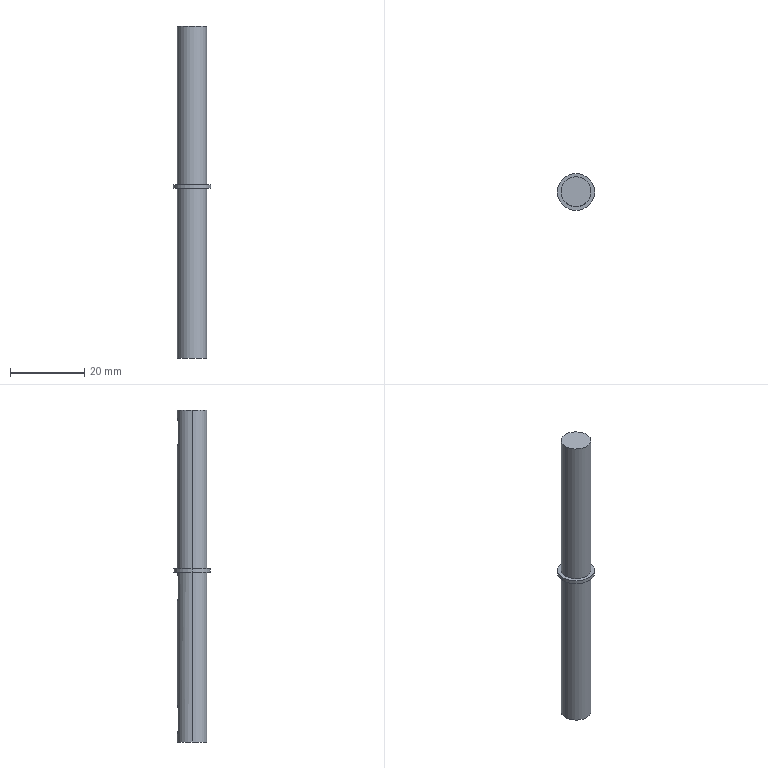Part | SolidWorks | features ICE 3, Extrusion 1 | 1 solid | 28 faces | box 10 x 10 x 89.39 mm | volume 4408 mm3 | cylinder 15 | plane 13 | commonest cylinder face diameters 3 x9 8 x4 10 x2
STEP:
#1=CARTESIAN_POINT('',(0.,2.2,10.));
#2=VERTEX_POINT('',#1);
#3=CARTESIAN_POINT('',(1.5,2.2,8.5));
#4=VERTEX_POINT('',#3);
#5=CARTESIAN_POINT('',(0.,2.2,8.5));
#6=DIRECTION('',(0.,1.,0.));
#7=DIRECTION('',(0.,0.,1.));
#8=AXIS2_PLACEMENT_3D('',#5,#6,#7);
#9=CIRCLE('',#8,1.5);
#10=EDGE_CURVE('',#2,#4,#9,.T.);
#11=ORIENTED_EDGE('',*,*,#10,.F.);
#12=CARTESIAN_POINT('',(0.,4.,10.));
#13=VERTEX_POINT('',#12);
#14=CARTESIAN_POINT('',(0.,2.2,10.));
#15=DIRECTION('',(0.,1.,0.));
#16=VECTOR('',#15,1000.);
#17=LINE('',#14,#16);
#18=EDGE_CURVE('',#2,#13,#17,.T.);
#19=ORIENTED_EDGE('',*,*,#18,.T.);
#20=CARTESIAN_POINT('',(1.5,3.708,8.5));
#21=VERTEX_POINT('',#20);
#22=CARTESIAN_POINT('',(1.5,3.708,8.5));
#23=CARTESIAN_POINT('',(1.5,3.708,8.6));
#24=CARTESIAN_POINT('',(1.49,3.712,8.698));
#25=CARTESIAN_POINT('',(1.451,3.727,8.891));
#26=CARTESIAN_POINT('',(1.422,3.739,8.987));
#27=CARTESIAN_POINT('',(1.309,3.781,9.259));
#28=CARTESIAN_POINT('',(1.197,3.819,9.424));
#29=CARTESIAN_POINT('',(0.9232,3.895,9.698));
#30=CARTESIAN_POINT('',(0.7573,3.932,9.809));
#31=CARTESIAN_POINT('',(0.4867,3.971,9.922));
#32=CARTESIAN_POINT('',(0.3912,3.982,9.951));
#33=CARTESIAN_POINT('',(0.197,3.996,9.99));
#34=CARTESIAN_POINT('',(0.09895,4.,10.));
#35=CARTESIAN_POINT('',(0.,4.,10.));
#36=B_SPLINE_CURVE_WITH_KNOTS('',3,(#22,#23,#24,#25,#26,#27,#28,#29,#30,#31,#32,#33,#34,#35),.UNSPECIFIED.,.F.,.F.,(4,2,2,2,2,2,4),(0.,0.0002959,0.0005918,0.001184,0.001775,0.002071,0.002367),.UNSPECIFIED.);
#37=EDGE_CURVE('',#21,#13,#36,.T.);
#38=ORIENTED_EDGE('',*,*,#37,.F.);
#39=CARTESIAN_POINT('',(1.5,2.2,8.5));
#40=DIRECTION('',(0.,1.,0.));
#41=VECTOR('',#40,1000.);
#42=LINE('',#39,#41);
#43=EDGE_CURVE('',#4,#21,#42,.T.);
#44=ORIENTED_EDGE('',*,*,#43,.F.);
#45=EDGE_LOOP('',(#11,#19,#38,#44));
#46=FACE_OUTER_BOUND('',#45,.T.);
#47=CARTESIAN_POINT('',(0.,2.2,8.5));
#48=DIRECTION('',(0.,1.,0.));
#49=DIRECTION('',(0.,0.,1.));
#50=AXIS2_PLACEMENT_3D('',#47,#48,#49);
#51=CYLINDRICAL_SURFACE('',#50,1.5);
#52=ADVANCED_FACE('',(#46),#51,.F.);
#53=CARTESIAN_POINT('',(0.,2.2,45.65));
#54=VERTEX_POINT('',#53);
#55=CARTESIAN_POINT('',(1.5,2.2,44.15));
#56=VERTEX_POINT('',#55);
#57=CARTESIAN_POINT('',(0.,2.2,44.15));
#58=DIRECTION('',(0.,1.,0.));
#59=DIRECTION('',(0.,0.,1.));
#60=AXIS2_PLACEMENT_3D('',#57,#58,#59);
#61=CIRCLE('',#60,1.5);
#62=EDGE_CURVE('',#54,#56,#61,.T.);
#63=ORIENTED_EDGE('',*,*,#62,.F.);
#64=CARTESIAN_POINT('',(0.,4.,45.65));
#65=VERTEX_POINT('',#64);
#66=CARTESIAN_POINT('',(0.,2.2,45.65));
#67=DIRECTION('',(0.,1.,0.));
#68=VECTOR('',#67,1000.);
#69=LINE('',#66,#68);
#70=EDGE_CURVE('',#54,#65,#69,.T.);
#71=ORIENTED_EDGE('',*,*,#70,.T.);
#72=CARTESIAN_POINT('',(1.5,3.708,44.15));
#73=VERTEX_POINT('',#72);
#74=CARTESIAN_POINT('',(1.5,3.708,44.15));
#75=CARTESIAN_POINT('',(1.5,3.708,44.25));
#76=CARTESIAN_POINT('',(1.49,3.712,44.348));
#77=CARTESIAN_POINT('',(1.451,3.727,44.541));
#78=CARTESIAN_POINT('',(1.422,3.739,44.637));
#79=CARTESIAN_POINT('',(1.309,3.781,44.909));
#80=CARTESIAN_POINT('',(1.197,3.819,45.074));
#81=CARTESIAN_POINT('',(0.9232,3.895,45.348));
#82=CARTESIAN_POINT('',(0.7573,3.932,45.459));
#83=CARTESIAN_POINT('',(0.4867,3.971,45.572));
#84=CARTESIAN_POINT('',(0.3912,3.982,45.601));
#85=CARTESIAN_POINT('',(0.197,3.996,45.64));
#86=CARTESIAN_POINT('',(0.09895,4.,45.65));
#87=CARTESIAN_POINT('',(0.,4.,45.65));
#88=B_SPLINE_CURVE_WITH_KNOTS('',3,(#74,#75,#76,#77,#78,#79,#80,#81,#82,#83,#84,#85,#86,#87),.UNSPECIFIED.,.F.,.F.,(4,2,2,2,2,2,4),(0.,0.0002959,0.0005918,0.001184,0.001775,0.002071,0.002367),.UNSPECIFIED.);
#89=EDGE_CURVE('',#73,#65,#88,.T.);
#90=ORIENTED_EDGE('',*,*,#89,.F.);
#91=CARTESIAN_POINT('',(1.5,2.2,44.15));
#92=DIRECTION('',(0.,1.,0.));
#93=VECTOR('',#92,1000.);
#94=LINE('',#91,#93);
#95=EDGE_CURVE('',#56,#73,#94,.T.);
#96=ORIENTED_EDGE('',*,*,#95,.F.);
#97=EDGE_LOOP('',(#63,#71,#90,#96));
#98=FACE_OUTER_BOUND('',#97,.T.);
#99=CARTESIAN_POINT('',(0.,2.2,44.15));
#100=DIRECTION('',(0.,1.,0.));
#101=DIRECTION('',(0.,0.,1.));
#102=AXIS2_PLACEMENT_3D('',#99,#100,#101);
#103=CYLINDRICAL_SURFACE('',#102,1.5);
#104=ADVANCED_FACE('',(#98),#103,.F.);
#105=CARTESIAN_POINT('',(0.,2.2,87.39));
#106=VERTEX_POINT('',#105);
#107=CARTESIAN_POINT('',(1.5,2.2,85.89));
#108=VERTEX_POINT('',#107);
#109=CARTESIAN_POINT('',(0.,2.2,85.89));
#110=DIRECTION('',(0.,1.,0.));
#111=DIRECTION('',(0.,0.,1.));
#112=AXIS2_PLACEMENT_3D('',#109,#110,#111);
#113=CIRCLE('',#112,1.5);
#114=EDGE_CURVE('',#106,#108,#113,.T.);
#115=ORIENTED_EDGE('',*,*,#114,.F.);
#116=CARTESIAN_POINT('',(0.,4.,87.39));
#117=VERTEX_POINT('',#116);
#118=CARTESIAN_POINT('',(0.,2.2,87.39));
#119=DIRECTION('',(0.,1.,0.));
#120=VECTOR('',#119,1000.);
#121=LINE('',#118,#120);
#122=EDGE_CURVE('',#106,#117,#121,.T.);
#123=ORIENTED_EDGE('',*,*,#122,.T.);
#124=CARTESIAN_POINT('',(1.5,3.708,85.89));
#125=VERTEX_POINT('',#124);
#126=CARTESIAN_POINT('',(1.5,3.708,85.89));
#127=CARTESIAN_POINT('',(1.5,3.708,85.99));
#128=CARTESIAN_POINT('',(1.49,3.712,86.088));
#129=CARTESIAN_POINT('',(1.451,3.727,86.281));
#130=CARTESIAN_POINT('',(1.422,3.739,86.377));
#131=CARTESIAN_POINT('',(1.309,3.781,86.649));
#132=CARTESIAN_POINT('',(1.197,3.819,86.814));
#133=CARTESIAN_POINT('',(0.9232,3.895,87.088));
#134=CARTESIAN_POINT('',(0.7573,3.932,87.199));
#135=CARTESIAN_POINT('',(0.4867,3.971,87.312));
#136=CARTESIAN_POINT('',(0.3912,3.982,87.341));
#137=CARTESIAN_POINT('',(0.197,3.996,87.38));
#138=CARTESIAN_POINT('',(0.09895,4.,87.39));
#139=CARTESIAN_POINT('',(0.,4.,87.39));
#140=B_SPLINE_CURVE_WITH_KNOTS('',3,(#126,#127,#128,#129,#130,#131,#132,#133,#134,#135,#136,#137,#138,#139),.UNSPECIFIED.,.F.,.F.,(4,2,2,2,2,2,4),(0.,0.0002959,0.0005918,0.001184,0.001775,0.002071,0.002367),.UNSPECIFIED.);
#141=EDGE_CURVE('',#125,#117,#140,.T.);
#142=ORIENTED_EDGE('',*,*,#141,.F.);
#143=CARTESIAN_POINT('',(1.5,2.2,85.89));
#144=DIRECTION('',(0.,1.,0.));
#145=VECTOR('',#144,1000.);
#146=LINE('',#143,#145);
#147=EDGE_CURVE('',#108,#125,#146,.T.);
#148=ORIENTED_EDGE('',*,*,#147,.F.);
#149=EDGE_LOOP('',(#115,#123,#142,#148));
#150=FACE_OUTER_BOUND('',#149,.T.);
#151=CARTESIAN_POINT('',(0.,2.2,85.89));
#152=DIRECTION('',(0.,1.,0.));
#153=DIRECTION('',(0.,0.,1.));
#154=AXIS2_PLACEMENT_3D('',#151,#152,#153);
#155=CYLINDRICAL_SURFACE('',#154,1.5);
#156=ADVANCED_FACE('',(#150),#155,.F.);
#157=CARTESIAN_POINT('',(1.5,3.708,80.89));
#158=VERTEX_POINT('',#157);
#159=CARTESIAN_POINT('',(1.5,3.708,89.39));
#160=DIRECTION('',(0.,0.,1.));
#161=VECTOR('',#160,1000.);
#162=LINE('',#159,#161);
#163=EDGE_CURVE('',#158,#125,#162,.T.);
#164=ORIENTED_EDGE('',*,*,#163,.T.);
#165=ORIENTED_EDGE('',*,*,#141,.T.);
#166=CARTESIAN_POINT('',(-1.5,3.708,85.89));
#167=VERTEX_POINT('',#166);
#168=CARTESIAN_POINT('',(0.,4.,87.39));
#169=CARTESIAN_POINT('',(-0.0988,4.,87.39));
#170=CARTESIAN_POINT('',(-0.1991,3.996,87.38));
#171=CARTESIAN_POINT('',(-0.3921,3.982,87.341));
#172=CARTESIAN_POINT('',(-0.486,3.971,87.313));
#173=CARTESIAN_POINT('',(-0.6687,3.945,87.236));
#174=CARTESIAN_POINT('',(-0.7547,3.929,87.19));
#175=CARTESIAN_POINT('',(-0.9162,3.895,87.082));
#176=CARTESIAN_POINT('',(-0.9924,3.876,87.019));
#177=CARTESIAN_POINT('',(-1.13,3.838,86.881));
#178=CARTESIAN_POINT('',(-1.191,3.819,86.807));
#179=CARTESIAN_POINT('',(-1.3,3.783,86.645));
#180=CARTESIAN_POINT('',(-1.347,3.767,86.558));
#181=CARTESIAN_POINT('',(-1.459,3.725,86.288));
#182=CARTESIAN_POINT('',(-1.5,3.708,86.09));
#183=CARTESIAN_POINT('',(-1.5,3.708,85.89));
#184=B_SPLINE_CURVE_WITH_KNOTS('',3,(#168,#169,#170,#171,#172,#173,#174,#175,#176,#177,#178,#179,#180,#181,#182,#183),.UNSPECIFIED.,.F.,.F.,(4,2,2,2,2,2,2,4),(0.002367,0.002663,0.002958,0.003254,0.003549,0.003845,0.00414,0.004731),.UNSPECIFIED.);
#185=EDGE_CURVE('',#117,#167,#184,.T.);
#186=ORIENTED_EDGE('',*,*,#185,.T.);
#187=CARTESIAN_POINT('',(-1.5,3.708,80.89));
#188=VERTEX_POINT('',#187);
#189=CARTESIAN_POINT('',(-1.5,3.708,89.39));
#190=DIRECTION('',(0.,0.,-1.));
#191=VECTOR('',#190,1000.);
#192=LINE('',#189,#191);
#193=EDGE_CURVE('',#167,#188,#192,.T.);
#194=ORIENTED_EDGE('',*,*,#193,.T.);
#195=CARTESIAN_POINT('',(-1.5,3.708,80.89));
#196=CARTESIAN_POINT('',(-1.5,3.708,80.79));
#197=CARTESIAN_POINT('',(-1.49,3.712,80.692));
#198=CARTESIAN_POINT('',(-1.451,3.727,80.499));
#199=CARTESIAN_POINT('',(-1.422,3.739,80.403));
#200=CARTESIAN_POINT('',(-1.309,3.781,80.132));
#201=CARTESIAN_POINT('',(-1.198,3.819,79.967));
#202=CARTESIAN_POINT('',(-0.924,3.894,79.693));
#203=CARTESIAN_POINT('',(-0.7582,3.932,79.581));
#204=CARTESIAN_POINT('',(-0.488,3.971,79.468));
#205=CARTESIAN_POINT('',(-0.3926,3.982,79.439));
#206=CARTESIAN_POINT('',(-0.1986,3.996,79.4));
#207=CARTESIAN_POINT('',(-0.1006,4.,79.39));
#208=CARTESIAN_POINT('',(0.09712,4.,79.39));
#209=CARTESIAN_POINT('',(0.1975,3.996,79.4));
#210=CARTESIAN_POINT('',(0.3907,3.982,79.438));
#211=CARTESIAN_POINT('',(0.4847,3.972,79.467));
#212=CARTESIAN_POINT('',(0.759,3.932,79.581));
#213=CARTESIAN_POINT('',(0.9229,3.895,79.692));
#214=CARTESIAN_POINT('',(1.129,3.838,79.898));
#215=CARTESIAN_POINT('',(1.191,3.819,79.973));
#216=CARTESIAN_POINT('',(1.299,3.783,80.134));
#217=CARTESIAN_POINT('',(1.347,3.767,80.222));
#218=CARTESIAN_POINT('',(1.459,3.725,80.492));
#219=CARTESIAN_POINT('',(1.5,3.708,80.69));
#220=CARTESIAN_POINT('',(1.5,3.708,80.89));
#221=B_SPLINE_CURVE_WITH_KNOTS('',3,(#195,#196,#197,#198,#199,#200,#201,#202,#203,#204,#205,#206,#207,#208,#209,#210,#211,#212,#213,#214,#215,#216,#217,#218,#219,#220),.UNSPECIFIED.,.F.,.F.,(4,2,2,2,2,2,2,2,2,2,2,2,4),(0.,0.0002957,0.0005914,0.001183,0.001774,0.00207,0.002366,0.002661,0.002957,0.003548,0.003844,0.00414,0.004731),.UNSPECIFIED.);
#222=EDGE_CURVE('',#188,#158,#221,.T.);
#223=ORIENTED_EDGE('',*,*,#222,.T.);
#224=EDGE_LOOP('',(#164,#165,#186,#194,#223));
#225=FACE_BOUND('',#224,.T.);
#226=CARTESIAN_POINT('',(4.,0.,89.39));
#227=VERTEX_POINT('',#226);
#228=CARTESIAN_POINT('',(-4.,0.,89.39));
#229=VERTEX_POINT('',#228);
#230=CARTESIAN_POINT('',(0.,0.,89.39));
#231=DIRECTION('',(0.,0.,1.));
#232=DIRECTION('',(1.,0.,0.));
#233=AXIS2_PLACEMENT_3D('',#230,#231,#232);
#234=CIRCLE('',#233,4.);
#235=EDGE_CURVE('',#227,#229,#234,.T.);
#236=ORIENTED_EDGE('',*,*,#235,.F.);
#237=CARTESIAN_POINT('',(4.,0.,46.65));
#238=VERTEX_POINT('',#237);
#239=CARTESIAN_POINT('',(4.,0.,89.39));
#240=DIRECTION('',(0.,0.,-1.));
#241=VECTOR('',#240,1000.);
#242=LINE('',#239,#241);
#243=EDGE_CURVE('',#227,#238,#242,.T.);
#244=ORIENTED_EDGE('',*,*,#243,.T.);
#245=CARTESIAN_POINT('',(-4.,0.,46.65));
#246=VERTEX_POINT('',#245);
#247=CARTESIAN_POINT('',(0.,0.,46.65));
#248=DIRECTION('',(0.,0.,1.));
#249=DIRECTION('',(1.,0.,0.));
#250=AXIS2_PLACEMENT_3D('',#247,#248,#249);
#251=CIRCLE('',#250,4.);
#252=EDGE_CURVE('',#238,#246,#251,.T.);
#253=ORIENTED_EDGE('',*,*,#252,.T.);
#254=CARTESIAN_POINT('',(-4.,0.,89.39));
#255=DIRECTION('',(0.,0.,-1.));
#256=VECTOR('',#255,1000.);
#257=LINE('',#254,#256);
#258=EDGE_CURVE('',#229,#246,#257,.T.);
#259=ORIENTED_EDGE('',*,*,#258,.F.);
#260=EDGE_LOOP('',(#236,#244,#253,#259));
#261=FACE_OUTER_BOUND('',#260,.T.);
#262=CARTESIAN_POINT('',(0.,0.,89.39));
#263=DIRECTION('',(0.,0.,-1.));
#264=DIRECTION('',(-1.,0.,0.));
#265=AXIS2_PLACEMENT_3D('',#262,#263,#264);
#266=CYLINDRICAL_SURFACE('',#265,4.);
#267=ADVANCED_FACE('',(#225,#261),#266,.T.);
#268=CARTESIAN_POINT('',(5.,0.,46.65));
#269=VERTEX_POINT('',#268);
#270=CARTESIAN_POINT('',(-5.,0.,46.65));
#271=VERTEX_POINT('',#270);
#272=CARTESIAN_POINT('',(0.,0.,46.65));
#273=DIRECTION('',(0.,0.,1.));
#274=DIRECTION('',(1.,0.,0.));
#275=AXIS2_PLACEMENT_3D('',#272,#273,#274);
#276=CIRCLE('',#275,5.);
#277=EDGE_CURVE('',#269,#271,#276,.T.);
#278=ORIENTED_EDGE('',*,*,#277,.F.);
#279=CARTESIAN_POINT('',(5.,0.,45.65));
#280=VERTEX_POINT('',#279);
#281=CARTESIAN_POINT('',(5.,0.,46.65));
#282=DIRECTION('',(0.,0.,-1.));
#283=VECTOR('',#282,1000.);
#284=LINE('',#281,#283);
#285=EDGE_CURVE('',#269,#280,#284,.T.);
#286=ORIENTED_EDGE('',*,*,#285,.T.);
#287=CARTESIAN_POINT('',(-5.,0.,45.65));
#288=VERTEX_POINT('',#287);
#289=CARTESIAN_POINT('',(0.,0.,45.65));
#290=DIRECTION('',(0.,0.,1.));
#291=DIRECTION('',(1.,0.,0.));
#292=AXIS2_PLACEMENT_3D('',#289,#290,#291);
#293=CIRCLE('',#292,5.);
#294=EDGE_CURVE('',#280,#288,#293,.T.);
#295=ORIENTED_EDGE('',*,*,#294,.T.);
#296=CARTESIAN_POINT('',(-5.,0.,46.65));
#297=DIRECTION('',(0.,0.,-1.));
#298=VECTOR('',#297,1000.);
#299=LINE('',#296,#298);
#300=EDGE_CURVE('',#271,#288,#299,.T.);
#301=ORIENTED_EDGE('',*,*,#300,.F.);
#302=EDGE_LOOP('',(#278,#286,#295,#301));
#303=FACE_OUTER_BOUND('',#302,.T.);
#304=CARTESIAN_POINT('',(0.,0.,46.65));
#305=DIRECTION('',(0.,0.,-1.));
#306=DIRECTION('',(-1.,0.,0.));
#307=AXIS2_PLACEMENT_3D('',#304,#305,#306);
#308=CYLINDRICAL_SURFACE('',#307,5.);
#309=ADVANCED_FACE('',(#303),#308,.T.);
#310=CARTESIAN_POINT('',(1.5,3.708,3.5));
#311=VERTEX_POINT('',#310);
#312=CARTESIAN_POINT('',(1.5,3.708,45.65));
#313=DIRECTION('',(0.,0.,1.));
#314=VECTOR('',#313,1000.);
#315=LINE('',#312,#314);
#316=EDGE_CURVE('',#311,#21,#315,.T.);
#317=ORIENTED_EDGE('',*,*,#316,.T.);
#318=ORIENTED_EDGE('',*,*,#37,.T.);
#319=CARTESIAN_POINT('',(-1.5,3.708,8.5));
#320=VERTEX_POINT('',#319);
#321=CARTESIAN_POINT('',(0.,4.,10.));
#322=CARTESIAN_POINT('',(-0.0988,4.,10.));
#323=CARTESIAN_POINT('',(-0.1991,3.996,9.99));
#324=CARTESIAN_POINT('',(-0.3921,3.982,9.951));
#325=CARTESIAN_POINT('',(-0.486,3.971,9.923));
#326=CARTESIAN_POINT('',(-0.6687,3.945,9.846));
#327=CARTESIAN_POINT('',(-0.7547,3.929,9.8));
#328=CARTESIAN_POINT('',(-0.9162,3.895,9.692));
#329=CARTESIAN_POINT('',(-0.9924,3.876,9.629));
#330=CARTESIAN_POINT('',(-1.13,3.838,9.491));
#331=CARTESIAN_POINT('',(-1.191,3.819,9.417));
#332=CARTESIAN_POINT('',(-1.3,3.783,9.255));
#333=CARTESIAN_POINT('',(-1.347,3.767,9.168));
#334=CARTESIAN_POINT('',(-1.459,3.725,8.898));
#335=CARTESIAN_POINT('',(-1.5,3.708,8.7));
#336=CARTESIAN_POINT('',(-1.5,3.708,8.5));
#337=B_SPLINE_CURVE_WITH_KNOTS('',3,(#321,#322,#323,#324,#325,#326,#327,#328,#329,#330,#331,#332,#333,#334,#335,#336),.UNSPECIFIED.,.F.,.F.,(4,2,2,2,2,2,2,4),(0.002367,0.002663,0.002958,0.003254,0.003549,0.003845,0.00414,0.004731),.UNSPECIFIED.);
#338=EDGE_CURVE('',#13,#320,#337,.T.);
#339=ORIENTED_EDGE('',*,*,#338,.T.);
#340=CARTESIAN_POINT('',(-1.5,3.708,3.5));
#341=VERTEX_POINT('',#340);
#342=CARTESIAN_POINT('',(-1.5,3.708,45.65));
#343=DIRECTION('',(0.,0.,-1.));
#344=VECTOR('',#343,1000.);
#345=LINE('',#342,#344);
#346=EDGE_CURVE('',#320,#341,#345,.T.);
#347=ORIENTED_EDGE('',*,*,#346,.T.);
#348=CARTESIAN_POINT('',(-1.5,3.708,3.5));
#349=CARTESIAN_POINT('',(-1.5,3.708,3.4));
#350=CARTESIAN_POINT('',(-1.49,3.712,3.302));
#351=CARTESIAN_POINT('',(-1.451,3.727,3.109));
#352=CARTESIAN_POINT('',(-1.422,3.739,3.013));
#353=CARTESIAN_POINT('',(-1.309,3.781,2.742));
#354=CARTESIAN_POINT('',(-1.198,3.819,2.577));
#355=CARTESIAN_POINT('',(-0.924,3.894,2.303));
#356=CARTESIAN_POINT('',(-0.7582,3.932,2.191));
#357=CARTESIAN_POINT('',(-0.488,3.971,2.078));
#358=CARTESIAN_POINT('',(-0.3926,3.982,2.049));
#359=CARTESIAN_POINT('',(-0.1986,3.996,2.01));
#360=CARTESIAN_POINT('',(-0.1006,4.,2.));
#361=CARTESIAN_POINT('',(0.09712,4.,2.));
#362=CARTESIAN_POINT('',(0.1975,3.996,2.01));
#363=CARTESIAN_POINT('',(0.3907,3.982,2.048));
#364=CARTESIAN_POINT('',(0.4847,3.972,2.077));
#365=CARTESIAN_POINT('',(0.759,3.932,2.191));
#366=CARTESIAN_POINT('',(0.9229,3.895,2.302));
#367=CARTESIAN_POINT('',(1.129,3.838,2.508));
#368=CARTESIAN_POINT('',(1.191,3.819,2.583));
#369=CARTESIAN_POINT('',(1.299,3.783,2.744));
#370=CARTESIAN_POINT('',(1.347,3.767,2.832));
#371=CARTESIAN_POINT('',(1.459,3.725,3.102));
#372=CARTESIAN_POINT('',(1.5,3.708,3.3));
#373=CARTESIAN_POINT('',(1.5,3.708,3.5));
#374=B_SPLINE_CURVE_WITH_KNOTS('',3,(#348,#349,#350,#351,#352,#353,#354,#355,#356,#357,#358,#359,#360,#361,#362,#363,#364,#365,#366,#367,#368,#369,#370,#371,#372,#373),.UNSPECIFIED.,.F.,.F.,(4,2,2,2,2,2,2,2,2,2,2,2,4),(0.,0.0002957,0.0005914,0.001183,0.001774,0.00207,0.002366,0.002661,0.002957,0.003548,0.003844,0.00414,0.004731),.UNSPECIFIED.);
#375=EDGE_CURVE('',#341,#311,#374,.T.);
#376=ORIENTED_EDGE('',*,*,#375,.T.);
#377=EDGE_LOOP('',(#317,#318,#339,#347,#376));
#378=FACE_BOUND('',#377,.T.);
#379=CARTESIAN_POINT('',(4.,0.,45.65));
#380=VERTEX_POINT('',#379);
#381=CARTESIAN_POINT('',(0.,0.,45.65));
#382=DIRECTION('',(0.,0.,1.));
#383=DIRECTION('',(1.,0.,0.));
#384=AXIS2_PLACEMENT_3D('',#381,#382,#383);
#385=CIRCLE('',#384,4.);
#386=EDGE_CURVE('',#380,#65,#385,.T.);
#387=ORIENTED_EDGE('',*,*,#386,.F.);
#388=CARTESIAN_POINT('',(4.,0.,0.));
#389=VERTEX_POINT('',#388);
#390=CARTESIAN_POINT('',(4.,0.,45.65));
#391=DIRECTION('',(0.,0.,-1.));
#392=VECTOR('',#391,1000.);
#393=LINE('',#390,#392);
#394=EDGE_CURVE('',#380,#389,#393,.T.);
#395=ORIENTED_EDGE('',*,*,#394,.T.);
#396=CARTESIAN_POINT('',(-4.,0.,0.));
#397=VERTEX_POINT('',#396);
#398=CARTESIAN_POINT('',(0.,0.,0.));
#399=DIRECTION('',(0.,0.,1.));
#400=DIRECTION('',(1.,0.,0.));
#401=AXIS2_PLACEMENT_3D('',#398,#399,#400);
#402=CIRCLE('',#401,4.);
#403=EDGE_CURVE('',#389,#397,#402,.T.);
#404=ORIENTED_EDGE('',*,*,#403,.T.);
#405=CARTESIAN_POINT('',(-4.,0.,45.65));
#406=VERTEX_POINT('',#405);
#407=CARTESIAN_POINT('',(-4.,0.,45.65));
#408=DIRECTION('',(0.,0.,-1.));
#409=VECTOR('',#408,1000.);
#410=LINE('',#407,#409);
#411=EDGE_CURVE('',#406,#397,#410,.T.);
#412=ORIENTED_EDGE('',*,*,#411,.F.);
#413=CARTESIAN_POINT('',(0.,0.,45.65));
#414=DIRECTION('',(0.,0.,1.));
#415=DIRECTION('',(1.,0.,0.));
#416=AXIS2_PLACEMENT_3D('',#413,#414,#415);
#417=CIRCLE('',#416,4.);
#418=EDGE_CURVE('',#65,#406,#417,.T.);
#419=ORIENTED_EDGE('',*,*,#418,.F.);
#420=CARTESIAN_POINT('',(-1.5,3.708,44.15));
#421=VERTEX_POINT('',#420);
#422=CARTESIAN_POINT('',(0.,4.,45.65));
#423=CARTESIAN_POINT('',(-0.0988,4.,45.65));
#424=CARTESIAN_POINT('',(-0.1991,3.996,45.64));
#425=CARTESIAN_POINT('',(-0.3921,3.982,45.601));
#426=CARTESIAN_POINT('',(-0.486,3.971,45.573));
#427=CARTESIAN_POINT('',(-0.6687,3.945,45.496));
#428=CARTESIAN_POINT('',(-0.7547,3.929,45.45));
#429=CARTESIAN_POINT('',(-0.9162,3.895,45.342));
#430=CARTESIAN_POINT('',(-0.9924,3.876,45.279));
#431=CARTESIAN_POINT('',(-1.13,3.838,45.141));
#432=CARTESIAN_POINT('',(-1.191,3.819,45.067));
#433=CARTESIAN_POINT('',(-1.3,3.783,44.905));
#434=CARTESIAN_POINT('',(-1.347,3.767,44.818));
#435=CARTESIAN_POINT('',(-1.459,3.725,44.548));
#436=CARTESIAN_POINT('',(-1.5,3.708,44.35));
#437=CARTESIAN_POINT('',(-1.5,3.708,44.15));
#438=B_SPLINE_CURVE_WITH_KNOTS('',3,(#422,#423,#424,#425,#426,#427,#428,#429,#430,#431,#432,#433,#434,#435,#436,#437),.UNSPECIFIED.,.F.,.F.,(4,2,2,2,2,2,2,4),(0.002367,0.002663,0.002958,0.003254,0.003549,0.003845,0.00414,0.004731),.UNSPECIFIED.);
#439=EDGE_CURVE('',#65,#421,#438,.T.);
#440=ORIENTED_EDGE('',*,*,#439,.T.);
#441=CARTESIAN_POINT('',(-1.5,3.708,39.15));
#442=VERTEX_POINT('',#441);
#443=CARTESIAN_POINT('',(-1.5,3.708,45.65));
#444=DIRECTION('',(0.,0.,-1.));
#445=VECTOR('',#444,1000.);
#446=LINE('',#443,#445);
#447=EDGE_CURVE('',#421,#442,#446,.T.);
#448=ORIENTED_EDGE('',*,*,#447,.T.);
#449=CARTESIAN_POINT('',(1.5,3.708,39.15));
#450=VERTEX_POINT('',#449);
#451=CARTESIAN_POINT('',(-1.5,3.708,39.15));
#452=CARTESIAN_POINT('',(-1.5,3.708,39.05));
#453=CARTESIAN_POINT('',(-1.49,3.712,38.952));
#454=CARTESIAN_POINT('',(-1.451,3.727,38.759));
#455=CARTESIAN_POINT('',(-1.422,3.739,38.663));
#456=CARTESIAN_POINT('',(-1.309,3.781,38.392));
#457=CARTESIAN_POINT('',(-1.198,3.819,38.227));
#458=CARTESIAN_POINT('',(-0.924,3.894,37.953));
#459=CARTESIAN_POINT('',(-0.7582,3.932,37.841));
#460=CARTESIAN_POINT('',(-0.488,3.971,37.728));
#461=CARTESIAN_POINT('',(-0.3926,3.982,37.699));
#462=CARTESIAN_POINT('',(-0.1986,3.996,37.66));
#463=CARTESIAN_POINT('',(-0.1006,4.,37.65));
#464=CARTESIAN_POINT('',(0.09712,4.,37.65));
#465=CARTESIAN_POINT('',(0.1975,3.996,37.66));
#466=CARTESIAN_POINT('',(0.3907,3.982,37.698));
#467=CARTESIAN_POINT('',(0.4847,3.972,37.727));
#468=CARTESIAN_POINT('',(0.759,3.932,37.841));
#469=CARTESIAN_POINT('',(0.9229,3.895,37.952));
#470=CARTESIAN_POINT('',(1.129,3.838,38.158));
#471=CARTESIAN_POINT('',(1.191,3.819,38.233));
#472=CARTESIAN_POINT('',(1.299,3.783,38.394));
#473=CARTESIAN_POINT('',(1.347,3.767,38.482));
#474=CARTESIAN_POINT('',(1.459,3.725,38.752));
#475=CARTESIAN_POINT('',(1.5,3.708,38.95));
#476=CARTESIAN_POINT('',(1.5,3.708,39.15));
#477=B_SPLINE_CURVE_WITH_KNOTS('',3,(#451,#452,#453,#454,#455,#456,#457,#458,#459,#460,#461,#462,#463,#464,#465,#466,#467,#468,#469,#470,#471,#472,#473,#474,#475,#476),.UNSPECIFIED.,.F.,.F.,(4,2,2,2,2,2,2,2,2,2,2,2,4),(0.,0.0002957,0.0005914,0.001183,0.001774,0.00207,0.002366,0.002661,0.002957,0.003548,0.003844,0.00414,0.004731),.UNSPECIFIED.);
#478=EDGE_CURVE('',#442,#450,#477,.T.);
#479=ORIENTED_EDGE('',*,*,#478,.T.);
#480=CARTESIAN_POINT('',(1.5,3.708,45.65));
#481=DIRECTION('',(0.,0.,1.));
#482=VECTOR('',#481,1000.);
#483=LINE('',#480,#482);
#484=EDGE_CURVE('',#450,#73,#483,.T.);
#485=ORIENTED_EDGE('',*,*,#484,.T.);
#486=ORIENTED_EDGE('',*,*,#89,.T.);
#487=EDGE_LOOP('',(#387,#395,#404,#412,#419,#440,#448,#479,#485,#486));
#488=FACE_OUTER_BOUND('',#487,.T.);
#489=CARTESIAN_POINT('',(0.,0.,45.65));
#490=DIRECTION('',(0.,0.,-1.));
#491=DIRECTION('',(-1.,0.,0.));
#492=AXIS2_PLACEMENT_3D('',#489,#490,#491);
#493=CYLINDRICAL_SURFACE('',#492,4.);
#494=ADVANCED_FACE('',(#378,#488),#493,.T.);
#495=ORIENTED_EDGE('',*,*,#394,.F.);
#496=CARTESIAN_POINT('',(0.,0.,45.65));
#497=DIRECTION('',(0.,0.,1.));
#498=DIRECTION('',(1.,0.,0.));
#499=AXIS2_PLACEMENT_3D('',#496,#497,#498);
#500=CIRCLE('',#499,4.);
#501=EDGE_CURVE('',#406,#380,#500,.T.);
#502=ORIENTED_EDGE('',*,*,#501,.F.);
#503=ORIENTED_EDGE('',*,*,#411,.T.);
#504=CARTESIAN_POINT('',(0.,0.,0.));
#505=DIRECTION('',(0.,0.,1.));
#506=DIRECTION('',(1.,0.,0.));
#507=AXIS2_PLACEMENT_3D('',#504,#505,#506);
#508=CIRCLE('',#507,4.);
#509=EDGE_CURVE('',#397,#389,#508,.T.);
#510=ORIENTED_EDGE('',*,*,#509,.T.);
#511=EDGE_LOOP('',(#495,#502,#503,#510));
#512=FACE_OUTER_BOUND('',#511,.T.);
#513=CARTESIAN_POINT('',(0.,0.,45.65));
#514=DIRECTION('',(0.,0.,-1.));
#515=DIRECTION('',(-1.,0.,0.));
#516=AXIS2_PLACEMENT_3D('',#513,#514,#515);
#517=CYLINDRICAL_SURFACE('',#516,4.);
#518=ADVANCED_FACE('',(#512),#517,.T.);
#519=ORIENTED_EDGE('',*,*,#509,.F.);
#520=ORIENTED_EDGE('',*,*,#403,.F.);
#521=EDGE_LOOP('',(#519,#520));
#522=FACE_OUTER_BOUND('',#521,.T.);
#523=CARTESIAN_POINT('',(0.,0.,0.));
#524=DIRECTION('',(0.,0.,1.));
#525=DIRECTION('',(1.,0.,0.));
#526=AXIS2_PLACEMENT_3D('',#523,#524,#525);
#527=PLANE('',#526);
#528=ADVANCED_FACE('',(#522),#527,.F.);
#529=ORIENTED_EDGE('',*,*,#285,.F.);
#530=CARTESIAN_POINT('',(0.,0.,46.65));
#531=DIRECTION('',(0.,0.,1.));
#532=DIRECTION('',(1.,0.,0.));
#533=AXIS2_PLACEMENT_3D('',#530,#531,#532);
#534=CIRCLE('',#533,5.);
#535=EDGE_CURVE('',#271,#269,#534,.T.);
#536=ORIENTED_EDGE('',*,*,#535,.F.);
#537=ORIENTED_EDGE('',*,*,#300,.T.);
#538=CARTESIAN_POINT('',(0.,0.,45.65));
#539=DIRECTION('',(0.,0.,1.));
#540=DIRECTION('',(1.,0.,0.));
#541=AXIS2_PLACEMENT_3D('',#538,#539,#540);
#542=CIRCLE('',#541,5.);
#543=EDGE_CURVE('',#288,#280,#542,.T.);
#544=ORIENTED_EDGE('',*,*,#543,.T.);
#545=EDGE_LOOP('',(#529,#536,#537,#544));
#546=FACE_OUTER_BOUND('',#545,.T.);
#547=CARTESIAN_POINT('',(0.,0.,46.65));
#548=DIRECTION('',(0.,0.,-1.));
#549=DIRECTION('',(-1.,0.,0.));
#550=AXIS2_PLACEMENT_3D('',#547,#548,#549);
#551=CYLINDRICAL_SURFACE('',#550,5.);
#552=ADVANCED_FACE('',(#546),#551,.T.);
#553=CARTESIAN_POINT('',(0.,0.,46.65));
#554=DIRECTION('',(0.,0.,1.));
#555=DIRECTION('',(1.,0.,0.));
#556=AXIS2_PLACEMENT_3D('',#553,#554,#555);
#557=CIRCLE('',#556,4.);
#558=EDGE_CURVE('',#246,#238,#557,.T.);
#559=ORIENTED_EDGE('',*,*,#558,.F.);
#560=ORIENTED_EDGE('',*,*,#252,.F.);
#561=EDGE_LOOP('',(#559,#560));
#562=FACE_BOUND('',#561,.T.);
#563=ORIENTED_EDGE('',*,*,#535,.T.);
#564=ORIENTED_EDGE('',*,*,#277,.T.);
#565=EDGE_LOOP('',(#563,#564));
#566=FACE_OUTER_BOUND('',#565,.T.);
#567=CARTESIAN_POINT('',(0.,0.,46.65));
#568=DIRECTION('',(0.,0.,1.));
#569=DIRECTION('',(1.,0.,0.));
#570=AXIS2_PLACEMENT_3D('',#567,#568,#569);
#571=PLANE('',#570);
#572=ADVANCED_FACE('',(#562,#566),#571,.T.);
#573=ORIENTED_EDGE('',*,*,#418,.T.);
#574=ORIENTED_EDGE('',*,*,#501,.T.);
#575=ORIENTED_EDGE('',*,*,#386,.T.);
#576=EDGE_LOOP('',(#573,#574,#575));
#577=FACE_BOUND('',#576,.T.);
#578=ORIENTED_EDGE('',*,*,#543,.F.);
#579=ORIENTED_EDGE('',*,*,#294,.F.);
#580=EDGE_LOOP('',(#578,#579));
#581=FACE_OUTER_BOUND('',#580,.T.);
#582=CARTESIAN_POINT('',(0.,0.,45.65));
#583=DIRECTION('',(0.,0.,1.));
#584=DIRECTION('',(1.,0.,0.));
#585=AXIS2_PLACEMENT_3D('',#582,#583,#584);
#586=PLANE('',#585);
#587=ADVANCED_FACE('',(#577,#581),#586,.F.);
#588=ORIENTED_EDGE('',*,*,#243,.F.);
#589=CARTESIAN_POINT('',(0.,0.,89.39));
#590=DIRECTION('',(0.,0.,1.));
#591=DIRECTION('',(1.,0.,0.));
#592=AXIS2_PLACEMENT_3D('',#589,#590,#591);
#593=CIRCLE('',#592,4.);
#594=EDGE_CURVE('',#229,#227,#593,.T.);
#595=ORIENTED_EDGE('',*,*,#594,.F.);
#596=ORIENTED_EDGE('',*,*,#258,.T.);
#597=ORIENTED_EDGE('',*,*,#558,.T.);
#598=EDGE_LOOP('',(#588,#595,#596,#597));
#599=FACE_OUTER_BOUND('',#598,.T.);
#600=CARTESIAN_POINT('',(0.,0.,89.39));
#601=DIRECTION('',(0.,0.,-1.));
#602=DIRECTION('',(-1.,0.,0.));
#603=AXIS2_PLACEMENT_3D('',#600,#601,#602);
#604=CYLINDRICAL_SURFACE('',#603,4.);
#605=ADVANCED_FACE('',(#599),#604,.T.);
#606=ORIENTED_EDGE('',*,*,#594,.T.);
#607=ORIENTED_EDGE('',*,*,#235,.T.);
#608=EDGE_LOOP('',(#606,#607));
#609=FACE_OUTER_BOUND('',#608,.T.);
#610=CARTESIAN_POINT('',(0.,0.,89.39));
#611=DIRECTION('',(0.,0.,1.));
#612=DIRECTION('',(1.,0.,0.));
#613=AXIS2_PLACEMENT_3D('',#610,#611,#612);
#614=PLANE('',#613);
#615=ADVANCED_FACE('',(#609),#614,.T.);
#616=CARTESIAN_POINT('',(-1.5,2.2,80.89));
#617=VERTEX_POINT('',#616);
#618=CARTESIAN_POINT('',(-1.5,2.2,80.89));
#619=DIRECTION('',(0.,1.,0.));
#620=VECTOR('',#619,1000.);
#621=LINE('',#618,#620);
#622=EDGE_CURVE('',#617,#188,#621,.T.);
#623=ORIENTED_EDGE('',*,*,#622,.F.);
#624=CARTESIAN_POINT('',(1.5,2.2,80.89));
#625=VERTEX_POINT('',#624);
#626=CARTESIAN_POINT('',(0.,2.2,80.89));
#627=DIRECTION('',(0.,1.,0.));
#628=DIRECTION('',(0.,0.,1.));
#629=AXIS2_PLACEMENT_3D('',#626,#627,#628);
#630=CIRCLE('',#629,1.5);
#631=EDGE_CURVE('',#625,#617,#630,.T.);
#632=ORIENTED_EDGE('',*,*,#631,.F.);
#633=CARTESIAN_POINT('',(1.5,2.2,80.89));
#634=DIRECTION('',(0.,1.,0.));
#635=VECTOR('',#634,1000.);
#636=LINE('',#633,#635);
#637=EDGE_CURVE('',#625,#158,#636,.T.);
#638=ORIENTED_EDGE('',*,*,#637,.T.);
#639=ORIENTED_EDGE('',*,*,#222,.F.);
#640=EDGE_LOOP('',(#623,#632,#638,#639));
#641=FACE_OUTER_BOUND('',#640,.T.);
#642=CARTESIAN_POINT('',(0.,2.2,80.89));
#643=DIRECTION('',(0.,1.,0.));
#644=DIRECTION('',(0.,0.,1.));
#645=AXIS2_PLACEMENT_3D('',#642,#643,#644);
#646=CYLINDRICAL_SURFACE('',#645,1.5);
#647=ADVANCED_FACE('',(#641),#646,.F.);
#648=ORIENTED_EDGE('',*,*,#637,.F.);
#649=CARTESIAN_POINT('',(1.5,2.2,80.89));
#650=DIRECTION('',(0.,0.,-1.));
#651=VECTOR('',#650,1000.);
#652=LINE('',#649,#651);
#653=EDGE_CURVE('',#108,#625,#652,.T.);
#654=ORIENTED_EDGE('',*,*,#653,.F.);
#655=ORIENTED_EDGE('',*,*,#147,.T.);
#656=ORIENTED_EDGE('',*,*,#163,.F.);
#657=EDGE_LOOP('',(#648,#654,#655,#656));
#658=FACE_OUTER_BOUND('',#657,.T.);
#659=CARTESIAN_POINT('',(1.5,2.2,80.89));
#660=DIRECTION('',(1.,0.,0.));
#661=DIRECTION('',(0.,0.,-1.));
#662=AXIS2_PLACEMENT_3D('',#659,#660,#661);
#663=PLANE('',#662);
#664=ADVANCED_FACE('',(#658),#663,.F.);
#665=ORIENTED_EDGE('',*,*,#122,.F.);
#666=CARTESIAN_POINT('',(-1.5,2.2,85.89));
#667=VERTEX_POINT('',#666);
#668=CARTESIAN_POINT('',(0.,2.2,85.89));
#669=DIRECTION('',(0.,1.,0.));
#670=DIRECTION('',(0.,0.,1.));
#671=AXIS2_PLACEMENT_3D('',#668,#669,#670);
#672=CIRCLE('',#671,1.5);
#673=EDGE_CURVE('',#667,#106,#672,.T.);
#674=ORIENTED_EDGE('',*,*,#673,.F.);
#675=CARTESIAN_POINT('',(-1.5,2.2,85.89));
#676=DIRECTION('',(0.,1.,0.));
#677=VECTOR('',#676,1000.);
#678=LINE('',#675,#677);
#679=EDGE_CURVE('',#667,#167,#678,.T.);
#680=ORIENTED_EDGE('',*,*,#679,.T.);
#681=ORIENTED_EDGE('',*,*,#185,.F.);
#682=EDGE_LOOP('',(#665,#674,#680,#681));
#683=FACE_OUTER_BOUND('',#682,.T.);
#684=CARTESIAN_POINT('',(0.,2.2,85.89));
#685=DIRECTION('',(0.,1.,0.));
#686=DIRECTION('',(0.,0.,1.));
#687=AXIS2_PLACEMENT_3D('',#684,#685,#686);
#688=CYLINDRICAL_SURFACE('',#687,1.5);
#689=ADVANCED_FACE('',(#683),#688,.F.);
#690=ORIENTED_EDGE('',*,*,#679,.F.);
#691=CARTESIAN_POINT('',(-1.5,2.2,80.89));
#692=DIRECTION('',(0.,0.,1.));
#693=VECTOR('',#692,1000.);
#694=LINE('',#691,#693);
#695=EDGE_CURVE('',#617,#667,#694,.T.);
#696=ORIENTED_EDGE('',*,*,#695,.F.);
#697=ORIENTED_EDGE('',*,*,#622,.T.);
#698=ORIENTED_EDGE('',*,*,#193,.F.);
#699=EDGE_LOOP('',(#690,#696,#697,#698));
#700=FACE_OUTER_BOUND('',#699,.T.);
#701=CARTESIAN_POINT('',(-1.5,2.2,80.89));
#702=DIRECTION('',(-1.,0.,0.));
#703=DIRECTION('',(0.,0.,1.));
#704=AXIS2_PLACEMENT_3D('',#701,#702,#703);
#705=PLANE('',#704);
#706=ADVANCED_FACE('',(#700),#705,.F.);
#707=ORIENTED_EDGE('',*,*,#631,.T.);
#708=ORIENTED_EDGE('',*,*,#695,.T.);
#709=ORIENTED_EDGE('',*,*,#673,.T.);
#710=ORIENTED_EDGE('',*,*,#114,.T.);
#711=ORIENTED_EDGE('',*,*,#653,.T.);
#712=EDGE_LOOP('',(#707,#708,#709,#710,#711));
#713=FACE_OUTER_BOUND('',#712,.T.);
#714=CARTESIAN_POINT('',(0.,2.2,80.89));
#715=DIRECTION('',(0.,1.,0.));
#716=DIRECTION('',(0.,0.,1.));
#717=AXIS2_PLACEMENT_3D('',#714,#715,#716);
#718=PLANE('',#717);
#719=ADVANCED_FACE('',(#713),#718,.T.);
#720=CARTESIAN_POINT('',(-1.5,2.2,39.15));
#721=VERTEX_POINT('',#720);
#722=CARTESIAN_POINT('',(-1.5,2.2,39.15));
#723=DIRECTION('',(0.,1.,0.));
#724=VECTOR('',#723,1000.);
#725=LINE('',#722,#724);
#726=EDGE_CURVE('',#721,#442,#725,.T.);
#727=ORIENTED_EDGE('',*,*,#726,.F.);
#728=CARTESIAN_POINT('',(1.5,2.2,39.15));
#729=VERTEX_POINT('',#728);
#730=CARTESIAN_POINT('',(0.,2.2,39.15));
#731=DIRECTION('',(0.,1.,0.));
#732=DIRECTION('',(0.,0.,1.));
#733=AXIS2_PLACEMENT_3D('',#730,#731,#732);
#734=CIRCLE('',#733,1.5);
#735=EDGE_CURVE('',#729,#721,#734,.T.);
#736=ORIENTED_EDGE('',*,*,#735,.F.);
#737=CARTESIAN_POINT('',(1.5,2.2,39.15));
#738=DIRECTION('',(0.,1.,0.));
#739=VECTOR('',#738,1000.);
#740=LINE('',#737,#739);
#741=EDGE_CURVE('',#729,#450,#740,.T.);
#742=ORIENTED_EDGE('',*,*,#741,.T.);
#743=ORIENTED_EDGE('',*,*,#478,.F.);
#744=EDGE_LOOP('',(#727,#736,#742,#743));
#745=FACE_OUTER_BOUND('',#744,.T.);
#746=CARTESIAN_POINT('',(0.,2.2,39.15));
#747=DIRECTION('',(0.,1.,0.));
#748=DIRECTION('',(0.,0.,1.));
#749=AXIS2_PLACEMENT_3D('',#746,#747,#748);
#750=CYLINDRICAL_SURFACE('',#749,1.5);
#751=ADVANCED_FACE('',(#745),#750,.F.);
#752=ORIENTED_EDGE('',*,*,#741,.F.);
#753=CARTESIAN_POINT('',(1.5,2.2,39.15));
#754=DIRECTION('',(0.,0.,-1.));
#755=VECTOR('',#754,1000.);
#756=LINE('',#753,#755);
#757=EDGE_CURVE('',#56,#729,#756,.T.);
#758=ORIENTED_EDGE('',*,*,#757,.F.);
#759=ORIENTED_EDGE('',*,*,#95,.T.);
#760=ORIENTED_EDGE('',*,*,#484,.F.);
#761=EDGE_LOOP('',(#752,#758,#759,#760));
#762=FACE_OUTER_BOUND('',#761,.T.);
#763=CARTESIAN_POINT('',(1.5,2.2,39.15));
#764=DIRECTION('',(1.,0.,0.));
#765=DIRECTION('',(0.,0.,-1.));
#766=AXIS2_PLACEMENT_3D('',#763,#764,#765);
#767=PLANE('',#766);
#768=ADVANCED_FACE('',(#762),#767,.F.);
#769=CARTESIAN_POINT('',(-1.5,2.2,44.15));
#770=VERTEX_POINT('',#769);
#771=CARTESIAN_POINT('',(-1.5,2.2,44.15));
#772=DIRECTION('',(0.,1.,0.));
#773=VECTOR('',#772,1000.);
#774=LINE('',#771,#773);
#775=EDGE_CURVE('',#770,#421,#774,.T.);
#776=ORIENTED_EDGE('',*,*,#775,.F.);
#777=CARTESIAN_POINT('',(-1.5,2.2,39.15));
#778=DIRECTION('',(0.,0.,1.));
#779=VECTOR('',#778,1000.);
#780=LINE('',#777,#779);
#781=EDGE_CURVE('',#721,#770,#780,.T.);
#782=ORIENTED_EDGE('',*,*,#781,.F.);
#783=ORIENTED_EDGE('',*,*,#726,.T.);
#784=ORIENTED_EDGE('',*,*,#447,.F.);
#785=EDGE_LOOP('',(#776,#782,#783,#784));
#786=FACE_OUTER_BOUND('',#785,.T.);
#787=CARTESIAN_POINT('',(-1.5,2.2,39.15));
#788=DIRECTION('',(-1.,0.,0.));
#789=DIRECTION('',(0.,0.,1.));
#790=AXIS2_PLACEMENT_3D('',#787,#788,#789);
#791=PLANE('',#790);
#792=ADVANCED_FACE('',(#786),#791,.F.);
#793=ORIENTED_EDGE('',*,*,#70,.F.);
#794=CARTESIAN_POINT('',(0.,2.2,44.15));
#795=DIRECTION('',(0.,1.,0.));
#796=DIRECTION('',(0.,0.,1.));
#797=AXIS2_PLACEMENT_3D('',#794,#795,#796);
#798=CIRCLE('',#797,1.5);
#799=EDGE_CURVE('',#770,#54,#798,.T.);
#800=ORIENTED_EDGE('',*,*,#799,.F.);
#801=ORIENTED_EDGE('',*,*,#775,.T.);
#802=ORIENTED_EDGE('',*,*,#439,.F.);
#803=EDGE_LOOP('',(#793,#800,#801,#802));
#804=FACE_OUTER_BOUND('',#803,.T.);
#805=CARTESIAN_POINT('',(0.,2.2,44.15));
#806=DIRECTION('',(0.,1.,0.));
#807=DIRECTION('',(0.,0.,1.));
#808=AXIS2_PLACEMENT_3D('',#805,#806,#807);
#809=CYLINDRICAL_SURFACE('',#808,1.5);
#810=ADVANCED_FACE('',(#804),#809,.F.);
#811=ORIENTED_EDGE('',*,*,#735,.T.);
#812=ORIENTED_EDGE('',*,*,#781,.T.);
#813=ORIENTED_EDGE('',*,*,#799,.T.);
#814=ORIENTED_EDGE('',*,*,#62,.T.);
#815=ORIENTED_EDGE('',*,*,#757,.T.);
#816=EDGE_LOOP('',(#811,#812,#813,#814,#815));
#817=FACE_OUTER_BOUND('',#816,.T.);
#818=CARTESIAN_POINT('',(0.,2.2,39.15));
#819=DIRECTION('',(0.,1.,0.));
#820=DIRECTION('',(0.,0.,1.));
#821=AXIS2_PLACEMENT_3D('',#818,#819,#820);
#822=PLANE('',#821);
#823=ADVANCED_FACE('',(#817),#822,.T.);
#824=CARTESIAN_POINT('',(-1.5,2.2,3.5));
#825=VERTEX_POINT('',#824);
#826=CARTESIAN_POINT('',(-1.5,2.2,3.5));
#827=DIRECTION('',(0.,1.,0.));
#828=VECTOR('',#827,1000.);
#829=LINE('',#826,#828);
#830=EDGE_CURVE('',#825,#341,#829,.T.);
#831=ORIENTED_EDGE('',*,*,#830,.F.);
#832=CARTESIAN_POINT('',(1.5,2.2,3.5));
#833=VERTEX_POINT('',#832);
#834=CARTESIAN_POINT('',(0.,2.2,3.5));
#835=DIRECTION('',(0.,1.,0.));
#836=DIRECTION('',(0.,0.,1.));
#837=AXIS2_PLACEMENT_3D('',#834,#835,#836);
#838=CIRCLE('',#837,1.5);
#839=EDGE_CURVE('',#833,#825,#838,.T.);
#840=ORIENTED_EDGE('',*,*,#839,.F.);
#841=CARTESIAN_POINT('',(1.5,2.2,3.5));
#842=DIRECTION('',(0.,1.,0.));
#843=VECTOR('',#842,1000.);
#844=LINE('',#841,#843);
#845=EDGE_CURVE('',#833,#311,#844,.T.);
#846=ORIENTED_EDGE('',*,*,#845,.T.);
#847=ORIENTED_EDGE('',*,*,#375,.F.);
#848=EDGE_LOOP('',(#831,#840,#846,#847));
#849=FACE_OUTER_BOUND('',#848,.T.);
#850=CARTESIAN_POINT('',(0.,2.2,3.5));
#851=DIRECTION('',(0.,1.,0.));
#852=DIRECTION('',(0.,0.,1.));
#853=AXIS2_PLACEMENT_3D('',#850,#851,#852);
#854=CYLINDRICAL_SURFACE('',#853,1.5);
#855=ADVANCED_FACE('',(#849),#854,.F.);
#856=ORIENTED_EDGE('',*,*,#845,.F.);
#857=CARTESIAN_POINT('',(1.5,2.2,3.5));
#858=DIRECTION('',(0.,0.,-1.));
#859=VECTOR('',#858,1000.);
#860=LINE('',#857,#859);
#861=EDGE_CURVE('',#4,#833,#860,.T.);
#862=ORIENTED_EDGE('',*,*,#861,.F.);
#863=ORIENTED_EDGE('',*,*,#43,.T.);
#864=ORIENTED_EDGE('',*,*,#316,.F.);
#865=EDGE_LOOP('',(#856,#862,#863,#864));
#866=FACE_OUTER_BOUND('',#865,.T.);
#867=CARTESIAN_POINT('',(1.5,2.2,3.5));
#868=DIRECTION('',(1.,0.,0.));
#869=DIRECTION('',(0.,0.,-1.));
#870=AXIS2_PLACEMENT_3D('',#867,#868,#869);
#871=PLANE('',#870);
#872=ADVANCED_FACE('',(#866),#871,.F.);
#873=ORIENTED_EDGE('',*,*,#18,.F.);
#874=CARTESIAN_POINT('',(-1.5,2.2,8.5));
#875=VERTEX_POINT('',#874);
#876=CARTESIAN_POINT('',(0.,2.2,8.5));
#877=DIRECTION('',(0.,1.,0.));
#878=DIRECTION('',(0.,0.,1.));
#879=AXIS2_PLACEMENT_3D('',#876,#877,#878);
#880=CIRCLE('',#879,1.5);
#881=EDGE_CURVE('',#875,#2,#880,.T.);
#882=ORIENTED_EDGE('',*,*,#881,.F.);
#883=CARTESIAN_POINT('',(-1.5,2.2,8.5));
#884=DIRECTION('',(0.,1.,0.));
#885=VECTOR('',#884,1000.);
#886=LINE('',#883,#885);
#887=EDGE_CURVE('',#875,#320,#886,.T.);
#888=ORIENTED_EDGE('',*,*,#887,.T.);
#889=ORIENTED_EDGE('',*,*,#338,.F.);
#890=EDGE_LOOP('',(#873,#882,#888,#889));
#891=FACE_OUTER_BOUND('',#890,.T.);
#892=CARTESIAN_POINT('',(0.,2.2,8.5));
#893=DIRECTION('',(0.,1.,0.));
#894=DIRECTION('',(0.,0.,1.));
#895=AXIS2_PLACEMENT_3D('',#892,#893,#894);
#896=CYLINDRICAL_SURFACE('',#895,1.5);
#897=ADVANCED_FACE('',(#891),#896,.F.);
#898=ORIENTED_EDGE('',*,*,#887,.F.);
#899=CARTESIAN_POINT('',(-1.5,2.2,3.5));
#900=DIRECTION('',(0.,0.,1.));
#901=VECTOR('',#900,1000.);
#902=LINE('',#899,#901);
#903=EDGE_CURVE('',#825,#875,#902,.T.);
#904=ORIENTED_EDGE('',*,*,#903,.F.);
#905=ORIENTED_EDGE('',*,*,#830,.T.);
#906=ORIENTED_EDGE('',*,*,#346,.F.);
#907=EDGE_LOOP('',(#898,#904,#905,#906));
#908=FACE_OUTER_BOUND('',#907,.T.);
#909=CARTESIAN_POINT('',(-1.5,2.2,3.5));
#910=DIRECTION('',(-1.,0.,0.));
#911=DIRECTION('',(0.,0.,1.));
#912=AXIS2_PLACEMENT_3D('',#909,#910,#911);
#913=PLANE('',#912);
#914=ADVANCED_FACE('',(#908),#913,.F.);
#915=ORIENTED_EDGE('',*,*,#839,.T.);
#916=ORIENTED_EDGE('',*,*,#903,.T.);
#917=ORIENTED_EDGE('',*,*,#881,.T.);
#918=ORIENTED_EDGE('',*,*,#10,.T.);
#919=ORIENTED_EDGE('',*,*,#861,.T.);
#920=EDGE_LOOP('',(#915,#916,#917,#918,#919));
#921=FACE_OUTER_BOUND('',#920,.T.);
#922=CARTESIAN_POINT('',(0.,2.2,3.5));
#923=DIRECTION('',(0.,1.,0.));
#924=DIRECTION('',(0.,0.,1.));
#925=AXIS2_PLACEMENT_3D('',#922,#923,#924);
#926=PLANE('',#925);
#927=ADVANCED_FACE('',(#921),#926,.T.);
#928=CLOSED_SHELL('',(#52,#104,#156,#267,#309,#494,#518,#528,#552,#572,#587,#605,#615,#647,#664,#689,#706,#719,#751,#768,#792,#810,#823,#855,#872,#897,#914,#927));
#929=MANIFOLD_SOLID_BREP('',#928);
#930=CARTESIAN_POINT('',(0.,0.,0.));
#931=DIRECTION('',(0.,0.,1.));
#932=DIRECTION('',(1.,0.,0.));
#933=AXIS2_PLACEMENT_3D('',#930,#931,#932);
#934=(LENGTH_UNIT()NAMED_UNIT(*)SI_UNIT(.MILLI.,.METRE.));
#935=UNCERTAINTY_MEASURE_WITH_UNIT(LENGTH_MEASURE(0.00001),#934,'','');
#936=(NAMED_UNIT(*)PLANE_ANGLE_UNIT()SI_UNIT($,.RADIAN.));
#937=(NAMED_UNIT(*)SI_UNIT($,.STERADIAN.)SOLID_ANGLE_UNIT());
#938=(GEOMETRIC_REPRESENTATION_CONTEXT(3)GLOBAL_UNCERTAINTY_ASSIGNED_CONTEXT((#935))GLOBAL_UNIT_ASSIGNED_CONTEXT((#934,#936,#937))REPRESENTATION_CONTEXT('',''));
#939=ADVANCED_BREP_SHAPE_REPRESENTATION('',(#929,#933),#938);